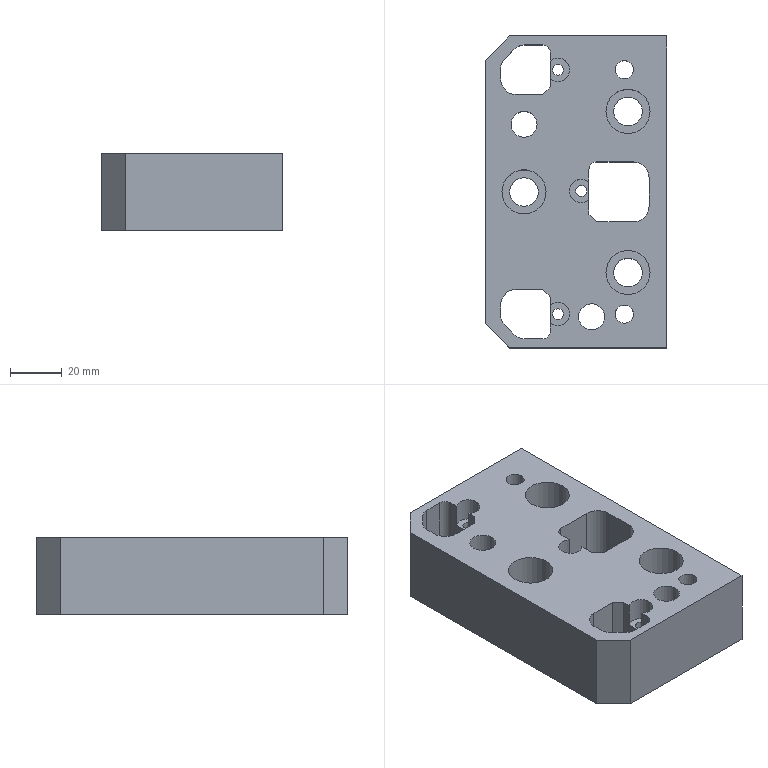Part | STEP file | 1 solid | 58 faces | box 70 x 120 x 30 mm | volume 188611 mm3 | plane 31 | cylinder 27 | commonest cylinder face diameters 10 x6 12 x4 4.2 x3 6 x3 9 x3 11 x3